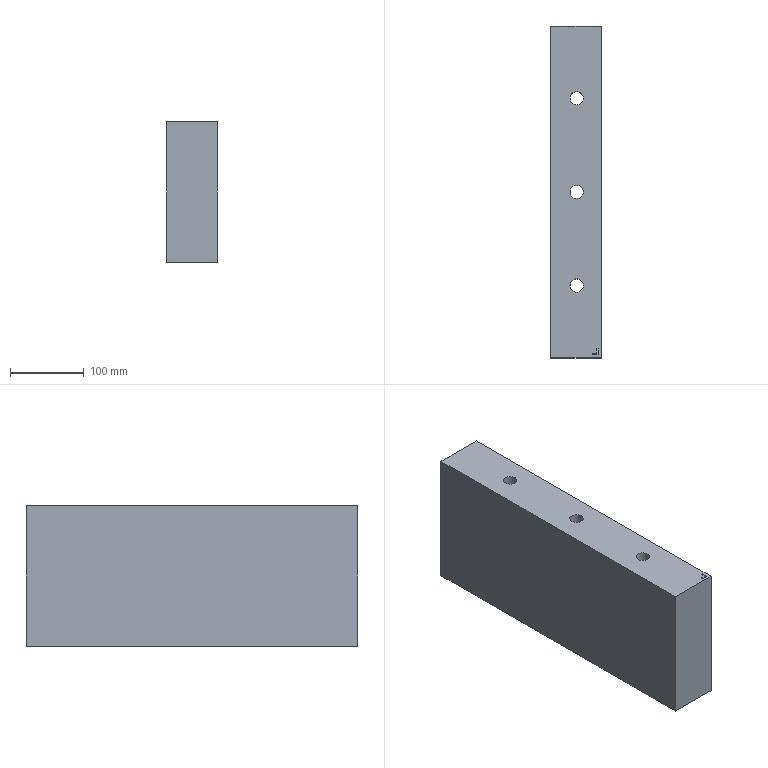Part | NX | features solid 2 | 1 solid | 32 faces | box 68 x 450 x 190 mm | volume 5663632 mm3 | plane 21 | cylinder 9 | cone 2 | commonest cylinder face diameters 18 x3 10.2 x2 11.7 x2 12 x2
STEP:
#1=CARTESIAN_POINT('',(-174.,127.,-380.5));
#2=VERTEX_POINT('',#1);
#3=CARTESIAN_POINT('',(-165.,127.,-380.5));
#4=DIRECTION('',(0.,0.,-1.));
#5=DIRECTION('',(-1.,0.,0.));
#6=AXIS2_PLACEMENT_3D('',#3,#4,#5);
#7=CIRCLE('',#6,9.);
#8=EDGE_CURVE('',#2,#2,#7,.T.);
#9=ORIENTED_EDGE('',*,*,#8,.F.);
#10=EDGE_LOOP('',(#9));
#11=FACE_BOUND('',#10,.T.);
#12=CARTESIAN_POINT('',(-174.,0.,-380.5));
#13=VERTEX_POINT('',#12);
#14=CARTESIAN_POINT('',(-165.,0.,-380.5));
#15=DIRECTION('',(0.,0.,-1.));
#16=DIRECTION('',(-1.,0.,0.));
#17=AXIS2_PLACEMENT_3D('',#14,#15,#16);
#18=CIRCLE('',#17,9.);
#19=EDGE_CURVE('',#13,#13,#18,.T.);
#20=ORIENTED_EDGE('',*,*,#19,.F.);
#21=EDGE_LOOP('',(#20));
#22=FACE_BOUND('',#21,.T.);
#23=CARTESIAN_POINT('',(-174.,-127.,-380.5));
#24=VERTEX_POINT('',#23);
#25=CARTESIAN_POINT('',(-165.,-127.,-380.5));
#26=DIRECTION('',(0.,0.,-1.));
#27=DIRECTION('',(-1.,0.,0.));
#28=AXIS2_PLACEMENT_3D('',#25,#26,#27);
#29=CIRCLE('',#28,9.);
#30=EDGE_CURVE('',#24,#24,#29,.T.);
#31=ORIENTED_EDGE('',*,*,#30,.F.);
#32=EDGE_LOOP('',(#31));
#33=FACE_BOUND('',#32,.T.);
#34=CARTESIAN_POINT('',(-170.1,187.,-380.5));
#35=VERTEX_POINT('',#34);
#36=CARTESIAN_POINT('',(-165.,187.,-380.5));
#37=DIRECTION('',(0.,0.,-1.));
#38=DIRECTION('',(-1.,0.,0.));
#39=AXIS2_PLACEMENT_3D('',#36,#37,#38);
#40=CIRCLE('',#39,5.1);
#41=EDGE_CURVE('',#35,#35,#40,.T.);
#42=ORIENTED_EDGE('',*,*,#41,.F.);
#43=EDGE_LOOP('',(#42));
#44=FACE_BOUND('',#43,.T.);
#45=CARTESIAN_POINT('',(-170.1,-187.,-380.5));
#46=VERTEX_POINT('',#45);
#47=CARTESIAN_POINT('',(-165.,-187.,-380.5));
#48=DIRECTION('',(0.,0.,-1.));
#49=DIRECTION('',(-1.,0.,0.));
#50=AXIS2_PLACEMENT_3D('',#47,#48,#49);
#51=CIRCLE('',#50,5.1);
#52=EDGE_CURVE('',#46,#46,#51,.T.);
#53=ORIENTED_EDGE('',*,*,#52,.F.);
#54=EDGE_LOOP('',(#53));
#55=FACE_BOUND('',#54,.T.);
#56=CARTESIAN_POINT('',(-132.,-225.,-380.5));
#57=VERTEX_POINT('',#56);
#58=CARTESIAN_POINT('',(-132.,225.,-380.5));
#59=VERTEX_POINT('',#58);
#60=CARTESIAN_POINT('',(-132.,0.,-380.5));
#61=DIRECTION('',(0.,1.,0.));
#62=VECTOR('',#61,1000.);
#63=LINE('',#60,#62);
#64=EDGE_CURVE('',#57,#59,#63,.T.);
#65=ORIENTED_EDGE('',*,*,#64,.F.);
#66=CARTESIAN_POINT('',(-200.,-225.,-380.5));
#67=VERTEX_POINT('',#66);
#68=CARTESIAN_POINT('',(-166.,-225.,-380.5));
#69=DIRECTION('',(1.,0.,0.));
#70=VECTOR('',#69,1000.);
#71=LINE('',#68,#70);
#72=EDGE_CURVE('',#67,#57,#71,.T.);
#73=ORIENTED_EDGE('',*,*,#72,.F.);
#74=CARTESIAN_POINT('',(-200.,225.,-380.5));
#75=VERTEX_POINT('',#74);
#76=CARTESIAN_POINT('',(-200.,0.,-380.5));
#77=DIRECTION('',(0.,-1.,0.));
#78=VECTOR('',#77,1000.);
#79=LINE('',#76,#78);
#80=EDGE_CURVE('',#75,#67,#79,.T.);
#81=ORIENTED_EDGE('',*,*,#80,.F.);
#82=CARTESIAN_POINT('',(-166.,225.,-380.5));
#83=DIRECTION('',(-1.,0.,0.));
#84=VECTOR('',#83,1000.);
#85=LINE('',#82,#84);
#86=EDGE_CURVE('',#59,#75,#85,.T.);
#87=ORIENTED_EDGE('',*,*,#86,.F.);
#88=EDGE_LOOP('',(#65,#73,#81,#87));
#89=FACE_BOUND('',#88,.T.);
#90=CARTESIAN_POINT('',(-165.,-192.85,-380.5));
#91=VERTEX_POINT('',#90);
#92=CARTESIAN_POINT('',(-159.15,-187.,-380.5));
#93=VERTEX_POINT('',#92);
#94=CARTESIAN_POINT('',(-165.,-187.,-380.5));
#95=DIRECTION('',(0.,0.,-1.));
#96=DIRECTION('',(-1.,0.,0.));
#97=AXIS2_PLACEMENT_3D('',#94,#95,#96);
#98=CIRCLE('',#97,5.85);
#99=EDGE_CURVE('',#91,#93,#98,.T.);
#100=ORIENTED_EDGE('',*,*,#99,.T.);
#101=CARTESIAN_POINT('',(-159.,-187.,-380.5));
#102=VERTEX_POINT('',#101);
#103=CARTESIAN_POINT('',(-166.,-187.,-380.5));
#104=DIRECTION('',(1.,0.,0.));
#105=VECTOR('',#104,1000.);
#106=LINE('',#103,#105);
#107=EDGE_CURVE('',#93,#102,#106,.T.);
#108=ORIENTED_EDGE('',*,*,#107,.T.);
#109=CARTESIAN_POINT('',(-165.,-193.,-380.5));
#110=VERTEX_POINT('',#109);
#111=CARTESIAN_POINT('',(-165.,-187.,-380.5));
#112=DIRECTION('',(0.,0.,-1.));
#113=DIRECTION('',(-1.,0.,0.));
#114=AXIS2_PLACEMENT_3D('',#111,#112,#113);
#115=CIRCLE('',#114,6.);
#116=EDGE_CURVE('',#110,#102,#115,.T.);
#117=ORIENTED_EDGE('',*,*,#116,.F.);
#118=CARTESIAN_POINT('',(-165.,0.,-380.5));
#119=DIRECTION('',(0.,1.,0.));
#120=VECTOR('',#119,1000.);
#121=LINE('',#118,#120);
#122=EDGE_CURVE('',#110,#91,#121,.T.);
#123=ORIENTED_EDGE('',*,*,#122,.T.);
#124=EDGE_LOOP('',(#100,#108,#117,#123));
#125=FACE_BOUND('',#124,.T.);
#126=CARTESIAN_POINT('',(-165.,181.15,-380.5));
#127=VERTEX_POINT('',#126);
#128=CARTESIAN_POINT('',(-159.15,187.,-380.5));
#129=VERTEX_POINT('',#128);
#130=CARTESIAN_POINT('',(-165.,187.,-380.5));
#131=DIRECTION('',(0.,0.,-1.));
#132=DIRECTION('',(-1.,0.,0.));
#133=AXIS2_PLACEMENT_3D('',#130,#131,#132);
#134=CIRCLE('',#133,5.85);
#135=EDGE_CURVE('',#127,#129,#134,.T.);
#136=ORIENTED_EDGE('',*,*,#135,.T.);
#137=CARTESIAN_POINT('',(-159.,187.,-380.5));
#138=VERTEX_POINT('',#137);
#139=CARTESIAN_POINT('',(-166.,187.,-380.5));
#140=DIRECTION('',(1.,0.,0.));
#141=VECTOR('',#140,1000.);
#142=LINE('',#139,#141);
#143=EDGE_CURVE('',#129,#138,#142,.T.);
#144=ORIENTED_EDGE('',*,*,#143,.T.);
#145=CARTESIAN_POINT('',(-165.,181.,-380.5));
#146=VERTEX_POINT('',#145);
#147=CARTESIAN_POINT('',(-165.,187.,-380.5));
#148=DIRECTION('',(0.,0.,-1.));
#149=DIRECTION('',(-1.,0.,0.));
#150=AXIS2_PLACEMENT_3D('',#147,#148,#149);
#151=CIRCLE('',#150,6.);
#152=EDGE_CURVE('',#146,#138,#151,.T.);
#153=ORIENTED_EDGE('',*,*,#152,.F.);
#154=CARTESIAN_POINT('',(-165.,0.,-380.5));
#155=DIRECTION('',(0.,1.,0.));
#156=VECTOR('',#155,1000.);
#157=LINE('',#154,#156);
#158=EDGE_CURVE('',#146,#127,#157,.T.);
#159=ORIENTED_EDGE('',*,*,#158,.T.);
#160=EDGE_LOOP('',(#136,#144,#153,#159));
#161=FACE_BOUND('',#160,.T.);
#162=CARTESIAN_POINT('',(-166.,0.,-380.5));
#163=DIRECTION('',(0.,0.,-1.));
#164=DIRECTION('',(-1.,0.,0.));
#165=AXIS2_PLACEMENT_3D('',#162,#163,#164);
#166=PLANE('',#165);
#167=ADVANCED_FACE('',(#11,#22,#33,#44,#55,#89,#125,#161),#166,.T.);
#168=CARTESIAN_POINT('',(-156.,127.,-190.5));
#169=VERTEX_POINT('',#168);
#170=CARTESIAN_POINT('',(-165.,127.,-190.5));
#171=DIRECTION('',(0.,0.,-1.));
#172=DIRECTION('',(1.,0.,0.));
#173=AXIS2_PLACEMENT_3D('',#170,#171,#172);
#174=CIRCLE('',#173,9.);
#175=EDGE_CURVE('',#169,#169,#174,.T.);
#176=ORIENTED_EDGE('',*,*,#175,.T.);
#177=EDGE_LOOP('',(#176));
#178=FACE_BOUND('',#177,.T.);
#179=CARTESIAN_POINT('',(-156.,0.,-190.5));
#180=VERTEX_POINT('',#179);
#181=CARTESIAN_POINT('',(-165.,0.,-190.5));
#182=DIRECTION('',(0.,0.,-1.));
#183=DIRECTION('',(1.,0.,0.));
#184=AXIS2_PLACEMENT_3D('',#181,#182,#183);
#185=CIRCLE('',#184,9.);
#186=EDGE_CURVE('',#180,#180,#185,.T.);
#187=ORIENTED_EDGE('',*,*,#186,.T.);
#188=EDGE_LOOP('',(#187));
#189=FACE_BOUND('',#188,.T.);
#190=CARTESIAN_POINT('',(-156.,-127.,-190.5));
#191=VERTEX_POINT('',#190);
#192=CARTESIAN_POINT('',(-165.,-127.,-190.5));
#193=DIRECTION('',(0.,0.,-1.));
#194=DIRECTION('',(1.,0.,0.));
#195=AXIS2_PLACEMENT_3D('',#192,#193,#194);
#196=CIRCLE('',#195,9.);
#197=EDGE_CURVE('',#191,#191,#196,.T.);
#198=ORIENTED_EDGE('',*,*,#197,.T.);
#199=EDGE_LOOP('',(#198));
#200=FACE_BOUND('',#199,.T.);
#201=CARTESIAN_POINT('',(-144.,-221.,-190.5));
#202=VERTEX_POINT('',#201);
#203=CARTESIAN_POINT('',(-136.,-221.,-190.5));
#204=VERTEX_POINT('',#203);
#205=CARTESIAN_POINT('',(-144.,-221.,-190.5));
#206=DIRECTION('',(1.,0.,0.));
#207=VECTOR('',#206,1000.);
#208=LINE('',#205,#207);
#209=EDGE_CURVE('',#202,#204,#208,.T.);
#210=ORIENTED_EDGE('',*,*,#209,.F.);
#211=CARTESIAN_POINT('',(-144.,-218.6,-190.5));
#212=VERTEX_POINT('',#211);
#213=CARTESIAN_POINT('',(-144.,-221.,-190.5));
#214=DIRECTION('',(0.,-1.,0.));
#215=VECTOR('',#214,1000.);
#216=LINE('',#213,#215);
#217=EDGE_CURVE('',#212,#202,#216,.T.);
#218=ORIENTED_EDGE('',*,*,#217,.F.);
#219=CARTESIAN_POINT('',(-138.4,-218.6,-190.5));
#220=VERTEX_POINT('',#219);
#221=CARTESIAN_POINT('',(-144.,-218.6,-190.5));
#222=DIRECTION('',(-1.,0.,0.));
#223=VECTOR('',#222,1000.);
#224=LINE('',#221,#223);
#225=EDGE_CURVE('',#220,#212,#224,.T.);
#226=ORIENTED_EDGE('',*,*,#225,.F.);
#227=CARTESIAN_POINT('',(-138.4,-213.,-190.5));
#228=VERTEX_POINT('',#227);
#229=CARTESIAN_POINT('',(-138.4,-218.6,-190.5));
#230=DIRECTION('',(0.,-1.,0.));
#231=VECTOR('',#230,1000.);
#232=LINE('',#229,#231);
#233=EDGE_CURVE('',#228,#220,#232,.T.);
#234=ORIENTED_EDGE('',*,*,#233,.F.);
#235=CARTESIAN_POINT('',(-136.,-213.,-190.5));
#236=VERTEX_POINT('',#235);
#237=CARTESIAN_POINT('',(-138.4,-213.,-190.5));
#238=DIRECTION('',(-1.,0.,0.));
#239=VECTOR('',#238,1000.);
#240=LINE('',#237,#239);
#241=EDGE_CURVE('',#236,#228,#240,.T.);
#242=ORIENTED_EDGE('',*,*,#241,.F.);
#243=CARTESIAN_POINT('',(-136.,-213.,-190.5));
#244=DIRECTION('',(0.,1.,0.));
#245=VECTOR('',#244,1000.);
#246=LINE('',#243,#245);
#247=EDGE_CURVE('',#204,#236,#246,.T.);
#248=ORIENTED_EDGE('',*,*,#247,.F.);
#249=EDGE_LOOP('',(#210,#218,#226,#234,#242,#248));
#250=FACE_BOUND('',#249,.T.);
#251=CARTESIAN_POINT('',(-132.,-225.,-190.5));
#252=VERTEX_POINT('',#251);
#253=CARTESIAN_POINT('',(-200.,-225.,-190.5));
#254=VERTEX_POINT('',#253);
#255=CARTESIAN_POINT('',(-166.,-225.,-190.5));
#256=DIRECTION('',(-1.,0.,0.));
#257=VECTOR('',#256,1000.);
#258=LINE('',#255,#257);
#259=EDGE_CURVE('',#252,#254,#258,.T.);
#260=ORIENTED_EDGE('',*,*,#259,.F.);
#261=CARTESIAN_POINT('',(-132.,225.,-190.5));
#262=VERTEX_POINT('',#261);
#263=CARTESIAN_POINT('',(-132.,0.,-190.5));
#264=DIRECTION('',(0.,-1.,0.));
#265=VECTOR('',#264,1000.);
#266=LINE('',#263,#265);
#267=EDGE_CURVE('',#262,#252,#266,.T.);
#268=ORIENTED_EDGE('',*,*,#267,.F.);
#269=CARTESIAN_POINT('',(-200.,225.,-190.5));
#270=VERTEX_POINT('',#269);
#271=CARTESIAN_POINT('',(-166.,225.,-190.5));
#272=DIRECTION('',(1.,0.,0.));
#273=VECTOR('',#272,1000.);
#274=LINE('',#271,#273);
#275=EDGE_CURVE('',#270,#262,#274,.T.);
#276=ORIENTED_EDGE('',*,*,#275,.F.);
#277=CARTESIAN_POINT('',(-200.,0.,-190.5));
#278=DIRECTION('',(0.,1.,0.));
#279=VECTOR('',#278,1000.);
#280=LINE('',#277,#279);
#281=EDGE_CURVE('',#254,#270,#280,.T.);
#282=ORIENTED_EDGE('',*,*,#281,.F.);
#283=EDGE_LOOP('',(#260,#268,#276,#282));
#284=FACE_BOUND('',#283,.T.);
#285=CARTESIAN_POINT('',(-166.,0.,-190.5));
#286=DIRECTION('',(0.,0.,1.));
#287=DIRECTION('',(1.,0.,0.));
#288=AXIS2_PLACEMENT_3D('',#285,#286,#287);
#289=PLANE('',#288);
#290=ADVANCED_FACE('',(#178,#189,#200,#250,#284),#289,.T.);
#291=CARTESIAN_POINT('',(-132.,-225.,-380.5));
#292=DIRECTION('',(0.,0.,1.));
#293=VECTOR('',#292,1000.);
#294=LINE('',#291,#293);
#295=EDGE_CURVE('',#57,#252,#294,.T.);
#296=ORIENTED_EDGE('',*,*,#295,.T.);
#297=ORIENTED_EDGE('',*,*,#259,.T.);
#298=CARTESIAN_POINT('',(-200.,-225.,-380.5));
#299=DIRECTION('',(0.,0.,1.));
#300=VECTOR('',#299,1000.);
#301=LINE('',#298,#300);
#302=EDGE_CURVE('',#67,#254,#301,.T.);
#303=ORIENTED_EDGE('',*,*,#302,.F.);
#304=ORIENTED_EDGE('',*,*,#72,.T.);
#305=EDGE_LOOP('',(#296,#297,#303,#304));
#306=FACE_BOUND('',#305,.T.);
#307=CARTESIAN_POINT('',(-166.,-225.,-380.5));
#308=DIRECTION('',(0.,-1.,0.));
#309=DIRECTION('',(0.,0.,-1.));
#310=AXIS2_PLACEMENT_3D('',#307,#308,#309);
#311=PLANE('',#310);
#312=ADVANCED_FACE('',(#306),#311,.T.);
#313=ORIENTED_EDGE('',*,*,#302,.T.);
#314=ORIENTED_EDGE('',*,*,#281,.T.);
#315=CARTESIAN_POINT('',(-200.,225.,-380.5));
#316=DIRECTION('',(0.,0.,1.));
#317=VECTOR('',#316,1000.);
#318=LINE('',#315,#317);
#319=EDGE_CURVE('',#75,#270,#318,.T.);
#320=ORIENTED_EDGE('',*,*,#319,.F.);
#321=ORIENTED_EDGE('',*,*,#80,.T.);
#322=EDGE_LOOP('',(#313,#314,#320,#321));
#323=FACE_BOUND('',#322,.T.);
#324=CARTESIAN_POINT('',(-200.,0.,-380.5));
#325=DIRECTION('',(-1.,0.,0.));
#326=DIRECTION('',(0.,0.,1.));
#327=AXIS2_PLACEMENT_3D('',#324,#325,#326);
#328=PLANE('',#327);
#329=ADVANCED_FACE('',(#323),#328,.T.);
#330=ORIENTED_EDGE('',*,*,#319,.T.);
#331=ORIENTED_EDGE('',*,*,#275,.T.);
#332=CARTESIAN_POINT('',(-132.,225.,-380.5));
#333=DIRECTION('',(0.,0.,1.));
#334=VECTOR('',#333,1000.);
#335=LINE('',#332,#334);
#336=EDGE_CURVE('',#59,#262,#335,.T.);
#337=ORIENTED_EDGE('',*,*,#336,.F.);
#338=ORIENTED_EDGE('',*,*,#86,.T.);
#339=EDGE_LOOP('',(#330,#331,#337,#338));
#340=FACE_BOUND('',#339,.T.);
#341=CARTESIAN_POINT('',(-166.,225.,-380.5));
#342=DIRECTION('',(0.,1.,0.));
#343=DIRECTION('',(0.,0.,1.));
#344=AXIS2_PLACEMENT_3D('',#341,#342,#343);
#345=PLANE('',#344);
#346=ADVANCED_FACE('',(#340),#345,.T.);
#347=ORIENTED_EDGE('',*,*,#64,.T.);
#348=ORIENTED_EDGE('',*,*,#336,.T.);
#349=ORIENTED_EDGE('',*,*,#267,.T.);
#350=ORIENTED_EDGE('',*,*,#295,.F.);
#351=EDGE_LOOP('',(#347,#348,#349,#350));
#352=FACE_BOUND('',#351,.T.);
#353=CARTESIAN_POINT('',(-132.,0.,-380.5));
#354=DIRECTION('',(1.,0.,0.));
#355=DIRECTION('',(0.,0.,-1.));
#356=AXIS2_PLACEMENT_3D('',#353,#354,#355);
#357=PLANE('',#356);
#358=ADVANCED_FACE('',(#352),#357,.T.);
#359=ORIENTED_EDGE('',*,*,#209,.T.);
#360=CARTESIAN_POINT('',(-136.,-221.,-190.8));
#361=VERTEX_POINT('',#360);
#362=CARTESIAN_POINT('',(-136.,-221.,-190.8));
#363=DIRECTION('',(0.,0.,1.));
#364=VECTOR('',#363,1000.);
#365=LINE('',#362,#364);
#366=EDGE_CURVE('',#361,#204,#365,.T.);
#367=ORIENTED_EDGE('',*,*,#366,.F.);
#368=CARTESIAN_POINT('',(-144.,-221.,-190.8));
#369=VERTEX_POINT('',#368);
#370=CARTESIAN_POINT('',(-144.,-221.,-190.8));
#371=DIRECTION('',(1.,0.,0.));
#372=VECTOR('',#371,1000.);
#373=LINE('',#370,#372);
#374=EDGE_CURVE('',#369,#361,#373,.T.);
#375=ORIENTED_EDGE('',*,*,#374,.F.);
#376=CARTESIAN_POINT('',(-144.,-221.,-190.8));
#377=DIRECTION('',(0.,0.,1.));
#378=VECTOR('',#377,1000.);
#379=LINE('',#376,#378);
#380=EDGE_CURVE('',#369,#202,#379,.T.);
#381=ORIENTED_EDGE('',*,*,#380,.T.);
#382=EDGE_LOOP('',(#359,#367,#375,#381));
#383=FACE_BOUND('',#382,.T.);
#384=CARTESIAN_POINT('',(-144.,-221.,-190.8));
#385=DIRECTION('',(0.,-1.,0.));
#386=DIRECTION('',(0.,0.,-1.));
#387=AXIS2_PLACEMENT_3D('',#384,#385,#386);
#388=PLANE('',#387);
#389=ADVANCED_FACE('',(#383),#388,.F.);
#390=ORIENTED_EDGE('',*,*,#247,.T.);
#391=CARTESIAN_POINT('',(-136.,-213.,-190.8));
#392=VERTEX_POINT('',#391);
#393=CARTESIAN_POINT('',(-136.,-213.,-190.8));
#394=DIRECTION('',(0.,0.,1.));
#395=VECTOR('',#394,1000.);
#396=LINE('',#393,#395);
#397=EDGE_CURVE('',#392,#236,#396,.T.);
#398=ORIENTED_EDGE('',*,*,#397,.F.);
#399=CARTESIAN_POINT('',(-136.,-213.,-190.8));
#400=DIRECTION('',(0.,1.,0.));
#401=VECTOR('',#400,1000.);
#402=LINE('',#399,#401);
#403=EDGE_CURVE('',#361,#392,#402,.T.);
#404=ORIENTED_EDGE('',*,*,#403,.F.);
#405=ORIENTED_EDGE('',*,*,#366,.T.);
#406=EDGE_LOOP('',(#390,#398,#404,#405));
#407=FACE_BOUND('',#406,.T.);
#408=CARTESIAN_POINT('',(-136.,-213.,-190.8));
#409=DIRECTION('',(1.,0.,0.));
#410=DIRECTION('',(0.,0.,-1.));
#411=AXIS2_PLACEMENT_3D('',#408,#409,#410);
#412=PLANE('',#411);
#413=ADVANCED_FACE('',(#407),#412,.F.);
#414=ORIENTED_EDGE('',*,*,#241,.T.);
#415=CARTESIAN_POINT('',(-138.4,-213.,-190.8));
#416=VERTEX_POINT('',#415);
#417=CARTESIAN_POINT('',(-138.4,-213.,-190.8));
#418=DIRECTION('',(0.,0.,1.));
#419=VECTOR('',#418,1000.);
#420=LINE('',#417,#419);
#421=EDGE_CURVE('',#416,#228,#420,.T.);
#422=ORIENTED_EDGE('',*,*,#421,.F.);
#423=CARTESIAN_POINT('',(-138.4,-213.,-190.8));
#424=DIRECTION('',(-1.,0.,0.));
#425=VECTOR('',#424,1000.);
#426=LINE('',#423,#425);
#427=EDGE_CURVE('',#392,#416,#426,.T.);
#428=ORIENTED_EDGE('',*,*,#427,.F.);
#429=ORIENTED_EDGE('',*,*,#397,.T.);
#430=EDGE_LOOP('',(#414,#422,#428,#429));
#431=FACE_BOUND('',#430,.T.);
#432=CARTESIAN_POINT('',(-138.4,-213.,-190.8));
#433=DIRECTION('',(0.,1.,0.));
#434=DIRECTION('',(0.,0.,1.));
#435=AXIS2_PLACEMENT_3D('',#432,#433,#434);
#436=PLANE('',#435);
#437=ADVANCED_FACE('',(#431),#436,.F.);
#438=ORIENTED_EDGE('',*,*,#233,.T.);
#439=CARTESIAN_POINT('',(-138.4,-218.6,-190.8));
#440=VERTEX_POINT('',#439);
#441=CARTESIAN_POINT('',(-138.4,-218.6,-190.8));
#442=DIRECTION('',(0.,0.,1.));
#443=VECTOR('',#442,1000.);
#444=LINE('',#441,#443);
#445=EDGE_CURVE('',#440,#220,#444,.T.);
#446=ORIENTED_EDGE('',*,*,#445,.F.);
#447=CARTESIAN_POINT('',(-138.4,-218.6,-190.8));
#448=DIRECTION('',(0.,-1.,0.));
#449=VECTOR('',#448,1000.);
#450=LINE('',#447,#449);
#451=EDGE_CURVE('',#416,#440,#450,.T.);
#452=ORIENTED_EDGE('',*,*,#451,.F.);
#453=ORIENTED_EDGE('',*,*,#421,.T.);
#454=EDGE_LOOP('',(#438,#446,#452,#453));
#455=FACE_BOUND('',#454,.T.);
#456=CARTESIAN_POINT('',(-138.4,-218.6,-190.8));
#457=DIRECTION('',(-1.,0.,0.));
#458=DIRECTION('',(0.,0.,1.));
#459=AXIS2_PLACEMENT_3D('',#456,#457,#458);
#460=PLANE('',#459);
#461=ADVANCED_FACE('',(#455),#460,.F.);
#462=ORIENTED_EDGE('',*,*,#225,.T.);
#463=CARTESIAN_POINT('',(-144.,-218.6,-190.8));
#464=VERTEX_POINT('',#463);
#465=CARTESIAN_POINT('',(-144.,-218.6,-190.8));
#466=DIRECTION('',(0.,0.,1.));
#467=VECTOR('',#466,1000.);
#468=LINE('',#465,#467);
#469=EDGE_CURVE('',#464,#212,#468,.T.);
#470=ORIENTED_EDGE('',*,*,#469,.F.);
#471=CARTESIAN_POINT('',(-144.,-218.6,-190.8));
#472=DIRECTION('',(-1.,0.,0.));
#473=VECTOR('',#472,1000.);
#474=LINE('',#471,#473);
#475=EDGE_CURVE('',#440,#464,#474,.T.);
#476=ORIENTED_EDGE('',*,*,#475,.F.);
#477=ORIENTED_EDGE('',*,*,#445,.T.);
#478=EDGE_LOOP('',(#462,#470,#476,#477));
#479=FACE_BOUND('',#478,.T.);
#480=CARTESIAN_POINT('',(-144.,-218.6,-190.8));
#481=DIRECTION('',(0.,1.,0.));
#482=DIRECTION('',(0.,0.,1.));
#483=AXIS2_PLACEMENT_3D('',#480,#481,#482);
#484=PLANE('',#483);
#485=ADVANCED_FACE('',(#479),#484,.F.);
#486=ORIENTED_EDGE('',*,*,#217,.T.);
#487=ORIENTED_EDGE('',*,*,#380,.F.);
#488=CARTESIAN_POINT('',(-144.,-221.,-190.8));
#489=DIRECTION('',(0.,-1.,0.));
#490=VECTOR('',#489,1000.);
#491=LINE('',#488,#490);
#492=EDGE_CURVE('',#464,#369,#491,.T.);
#493=ORIENTED_EDGE('',*,*,#492,.F.);
#494=ORIENTED_EDGE('',*,*,#469,.T.);
#495=EDGE_LOOP('',(#486,#487,#493,#494));
#496=FACE_BOUND('',#495,.T.);
#497=CARTESIAN_POINT('',(-144.,-221.,-190.8));
#498=DIRECTION('',(-1.,0.,0.));
#499=DIRECTION('',(0.,0.,1.));
#500=AXIS2_PLACEMENT_3D('',#497,#498,#499);
#501=PLANE('',#500);
#502=ADVANCED_FACE('',(#496),#501,.F.);
#503=ORIENTED_EDGE('',*,*,#374,.T.);
#504=ORIENTED_EDGE('',*,*,#403,.T.);
#505=ORIENTED_EDGE('',*,*,#427,.T.);
#506=ORIENTED_EDGE('',*,*,#451,.T.);
#507=ORIENTED_EDGE('',*,*,#475,.T.);
#508=ORIENTED_EDGE('',*,*,#492,.T.);
#509=EDGE_LOOP('',(#503,#504,#505,#506,#507,#508));
#510=FACE_BOUND('',#509,.T.);
#511=CARTESIAN_POINT('',(-136.,-221.,-190.8));
#512=DIRECTION('',(0.,0.,1.));
#513=DIRECTION('',(1.,0.,0.));
#514=AXIS2_PLACEMENT_3D('',#511,#512,#513);
#515=PLANE('',#514);
#516=ADVANCED_FACE('',(#510),#515,.T.);
#517=CARTESIAN_POINT('',(-159.9,-187.,-356.5));
#518=VERTEX_POINT('',#517);
#519=CARTESIAN_POINT('',(-165.,-192.1,-356.5));
#520=VERTEX_POINT('',#519);
#521=CARTESIAN_POINT('',(-165.,-187.,-356.5));
#522=DIRECTION('',(0.,0.,1.));
#523=DIRECTION('',(0.,-1.,0.));
#524=AXIS2_PLACEMENT_3D('',#521,#522,#523);
#525=CIRCLE('',#524,5.1);
#526=EDGE_CURVE('',#518,#520,#525,.T.);
#527=ORIENTED_EDGE('',*,*,#526,.T.);
#528=CARTESIAN_POINT('',(-165.,-193.,-356.5));
#529=VERTEX_POINT('',#528);
#530=CARTESIAN_POINT('',(-165.,-193.,-356.5));
#531=DIRECTION('',(0.,1.,0.));
#532=VECTOR('',#531,1000.);
#533=LINE('',#530,#532);
#534=EDGE_CURVE('',#529,#520,#533,.T.);
#535=ORIENTED_EDGE('',*,*,#534,.F.);
#536=CARTESIAN_POINT('',(-159.,-187.,-356.5));
#537=VERTEX_POINT('',#536);
#538=CARTESIAN_POINT('',(-165.,-187.,-356.5));
#539=DIRECTION('',(0.,0.,-1.));
#540=DIRECTION('',(1.,0.,0.));
#541=AXIS2_PLACEMENT_3D('',#538,#539,#540);
#542=CIRCLE('',#541,6.);
#543=EDGE_CURVE('',#529,#537,#542,.T.);
#544=ORIENTED_EDGE('',*,*,#543,.T.);
#545=CARTESIAN_POINT('',(-159.,-187.,-356.5));
#546=DIRECTION('',(1.,0.,0.));
#547=VECTOR('',#546,1000.);
#548=LINE('',#545,#547);
#549=EDGE_CURVE('',#518,#537,#548,.T.);
#550=ORIENTED_EDGE('',*,*,#549,.F.);
#551=EDGE_LOOP('',(#527,#535,#544,#550));
#552=FACE_BOUND('',#551,.T.);
#553=CARTESIAN_POINT('',(-165.,-187.,-356.5));
#554=DIRECTION('',(0.,0.,1.));
#555=DIRECTION('',(0.,-1.,0.));
#556=AXIS2_PLACEMENT_3D('',#553,#554,#555);
#557=PLANE('',#556);
#558=ADVANCED_FACE('',(#552),#557,.F.);
#559=ORIENTED_EDGE('',*,*,#116,.T.);
#560=CARTESIAN_POINT('',(-159.,-187.,-356.5));
#561=DIRECTION('',(0.,0.,-1.));
#562=VECTOR('',#561,1000.);
#563=LINE('',#560,#562);
#564=EDGE_CURVE('',#102,#537,#563,.F.);
#565=ORIENTED_EDGE('',*,*,#564,.T.);
#566=ORIENTED_EDGE('',*,*,#543,.F.);
#567=CARTESIAN_POINT('',(-165.,-193.,-356.5));
#568=DIRECTION('',(0.,0.,-1.));
#569=VECTOR('',#568,1000.);
#570=LINE('',#567,#569);
#571=EDGE_CURVE('',#529,#110,#570,.T.);
#572=ORIENTED_EDGE('',*,*,#571,.T.);
#573=EDGE_LOOP('',(#559,#565,#566,#572));
#574=FACE_BOUND('',#573,.T.);
#575=CARTESIAN_POINT('',(-165.,-187.,-356.5));
#576=DIRECTION('',(0.,0.,-1.));
#577=DIRECTION('',(1.,0.,0.));
#578=AXIS2_PLACEMENT_3D('',#575,#576,#577);
#579=CYLINDRICAL_SURFACE('',#578,6.);
#580=ADVANCED_FACE('',(#574),#579,.F.);
#581=CARTESIAN_POINT('',(-159.15,-187.,-357.5));
#582=VERTEX_POINT('',#581);
#583=CARTESIAN_POINT('',(-159.9,-187.,-357.5));
#584=VERTEX_POINT('',#583);
#585=CARTESIAN_POINT('',(-165.,-187.,-357.5));
#586=DIRECTION('',(-1.,0.,0.));
#587=VECTOR('',#586,1000.);
#588=LINE('',#585,#587);
#589=EDGE_CURVE('',#582,#584,#588,.T.);
#590=ORIENTED_EDGE('',*,*,#589,.F.);
#591=CARTESIAN_POINT('',(-165.,-192.85,-357.5));
#592=VERTEX_POINT('',#591);
#593=CARTESIAN_POINT('',(-165.,-187.,-357.5));
#594=DIRECTION('',(0.,0.,-1.));
#595=DIRECTION('',(1.,0.,0.));
#596=AXIS2_PLACEMENT_3D('',#593,#594,#595);
#597=CIRCLE('',#596,5.85);
#598=EDGE_CURVE('',#592,#582,#597,.T.);
#599=ORIENTED_EDGE('',*,*,#598,.F.);
#600=CARTESIAN_POINT('',(-165.,-192.1,-357.5));
#601=VERTEX_POINT('',#600);
#602=CARTESIAN_POINT('',(-165.,-187.,-357.5));
#603=DIRECTION('',(0.,-1.,0.));
#604=VECTOR('',#603,1000.);
#605=LINE('',#602,#604);
#606=EDGE_CURVE('',#601,#592,#605,.T.);
#607=ORIENTED_EDGE('',*,*,#606,.F.);
#608=CARTESIAN_POINT('',(-165.,-187.,-357.5));
#609=DIRECTION('',(0.,0.,1.));
#610=DIRECTION('',(0.,-1.,0.));
#611=AXIS2_PLACEMENT_3D('',#608,#609,#610);
#612=CIRCLE('',#611,5.1);
#613=EDGE_CURVE('',#584,#601,#612,.T.);
#614=ORIENTED_EDGE('',*,*,#613,.F.);
#615=EDGE_LOOP('',(#590,#599,#607,#614));
#616=FACE_BOUND('',#615,.T.);
#617=CARTESIAN_POINT('',(-165.,-187.,-357.5));
#618=DIRECTION('',(0.,0.,1.));
#619=DIRECTION('',(0.,-1.,0.));
#620=AXIS2_PLACEMENT_3D('',#617,#618,#619);
#621=PLANE('',#620);
#622=ADVANCED_FACE('',(#616),#621,.T.);
#623=CARTESIAN_POINT('',(-165.,-192.85,-357.5));
#624=DIRECTION('',(0.,0.,-1.));
#625=VECTOR('',#624,1000.);
#626=LINE('',#623,#625);
#627=EDGE_CURVE('',#592,#91,#626,.T.);
#628=ORIENTED_EDGE('',*,*,#627,.F.);
#629=ORIENTED_EDGE('',*,*,#598,.T.);
#630=CARTESIAN_POINT('',(-159.15,-187.,-357.5));
#631=DIRECTION('',(0.,0.,-1.));
#632=VECTOR('',#631,1000.);
#633=LINE('',#630,#632);
#634=EDGE_CURVE('',#93,#582,#633,.F.);
#635=ORIENTED_EDGE('',*,*,#634,.F.);
#636=ORIENTED_EDGE('',*,*,#99,.F.);
#637=EDGE_LOOP('',(#628,#629,#635,#636));
#638=FACE_BOUND('',#637,.T.);
#639=CARTESIAN_POINT('',(-165.,-187.,-357.5));
#640=DIRECTION('',(0.,0.,-1.));
#641=DIRECTION('',(1.,0.,0.));
#642=AXIS2_PLACEMENT_3D('',#639,#640,#641);
#643=CYLINDRICAL_SURFACE('',#642,5.85);
#644=ADVANCED_FACE('',(#638),#643,.T.);
#645=ORIENTED_EDGE('',*,*,#634,.T.);
#646=ORIENTED_EDGE('',*,*,#589,.T.);
#647=CARTESIAN_POINT('',(-159.9,-187.,-350.449));
#648=DIRECTION('',(0.,0.,-1.));
#649=VECTOR('',#648,1000.);
#650=LINE('',#647,#649);
#651=EDGE_CURVE('',#518,#584,#650,.T.);
#652=ORIENTED_EDGE('',*,*,#651,.F.);
#653=ORIENTED_EDGE('',*,*,#549,.T.);
#654=ORIENTED_EDGE('',*,*,#564,.F.);
#655=ORIENTED_EDGE('',*,*,#107,.F.);
#656=EDGE_LOOP('',(#645,#646,#652,#653,#654,#655));
#657=FACE_BOUND('',#656,.T.);
#658=CARTESIAN_POINT('',(-159.,-187.,-356.5));
#659=DIRECTION('',(0.,1.,0.));
#660=DIRECTION('',(0.,0.,1.));
#661=AXIS2_PLACEMENT_3D('',#658,#659,#660);
#662=PLANE('',#661);
#663=ADVANCED_FACE('',(#657),#662,.T.);
#664=ORIENTED_EDGE('',*,*,#571,.F.);
#665=ORIENTED_EDGE('',*,*,#534,.T.);
#666=CARTESIAN_POINT('',(-165.,-192.1,-350.449));
#667=DIRECTION('',(0.,0.,-1.));
#668=VECTOR('',#667,1000.);
#669=LINE('',#666,#668);
#670=EDGE_CURVE('',#601,#520,#669,.F.);
#671=ORIENTED_EDGE('',*,*,#670,.F.);
#672=ORIENTED_EDGE('',*,*,#606,.T.);
#673=ORIENTED_EDGE('',*,*,#627,.T.);
#674=ORIENTED_EDGE('',*,*,#122,.F.);
#675=EDGE_LOOP('',(#664,#665,#671,#672,#673,#674));
#676=FACE_BOUND('',#675,.T.);
#677=CARTESIAN_POINT('',(-165.,-193.,-356.5));
#678=DIRECTION('',(-1.,0.,0.));
#679=DIRECTION('',(0.,0.,1.));
#680=AXIS2_PLACEMENT_3D('',#677,#678,#679);
#681=PLANE('',#680);
#682=ADVANCED_FACE('',(#676),#681,.T.);
#683=ORIENTED_EDGE('',*,*,#52,.T.);
#684=EDGE_LOOP('',(#683));
#685=FACE_BOUND('',#684,.T.);
#686=CARTESIAN_POINT('',(-159.9,-187.,-350.449));
#687=VERTEX_POINT('',#686);
#688=CARTESIAN_POINT('',(-165.,-187.,-350.449));
#689=DIRECTION('',(0.,0.,1.));
#690=DIRECTION('',(1.,0.,0.));
#691=AXIS2_PLACEMENT_3D('',#688,#689,#690);
#692=CIRCLE('',#691,5.1);
#693=EDGE_CURVE('',#687,#687,#692,.T.);
#694=ORIENTED_EDGE('',*,*,#693,.T.);
#695=EDGE_LOOP('',(#694));
#696=FACE_BOUND('',#695,.T.);
#697=ORIENTED_EDGE('',*,*,#651,.T.);
#698=ORIENTED_EDGE('',*,*,#613,.T.);
#699=ORIENTED_EDGE('',*,*,#670,.T.);
#700=ORIENTED_EDGE('',*,*,#526,.F.);
#701=EDGE_LOOP('',(#697,#698,#699,#700));
#702=FACE_BOUND('',#701,.T.);
#703=CARTESIAN_POINT('',(-165.,-187.,-350.449));
#704=DIRECTION('',(0.,0.,-1.));
#705=DIRECTION('',(1.,0.,0.));
#706=AXIS2_PLACEMENT_3D('',#703,#704,#705);
#707=CYLINDRICAL_SURFACE('',#706,5.1);
#708=ADVANCED_FACE('',(#685,#696,#702),#707,.F.);
#709=ORIENTED_EDGE('',*,*,#693,.F.);
#710=EDGE_LOOP('',(#709));
#711=FACE_BOUND('',#710,.T.);
#712=CARTESIAN_POINT('',(-165.,-187.,-347.505));
#713=VERTEX_POINT('',#712);
#714=VERTEX_LOOP('',#713);
#715=FACE_BOUND('',#714,.T.);
#716=CARTESIAN_POINT('',(-165.,-187.,-347.505));
#717=DIRECTION('',(0.,0.,-1.));
#718=DIRECTION('',(1.,0.,0.));
#719=AXIS2_PLACEMENT_3D('',#716,#717,#718);
#720=CONICAL_SURFACE('',#719,0.,1.047);
#721=ADVANCED_FACE('',(#711,#715),#720,.F.);
#722=CARTESIAN_POINT('',(-159.9,187.,-356.5));
#723=VERTEX_POINT('',#722);
#724=CARTESIAN_POINT('',(-165.,181.9,-356.5));
#725=VERTEX_POINT('',#724);
#726=CARTESIAN_POINT('',(-165.,187.,-356.5));
#727=DIRECTION('',(0.,0.,1.));
#728=DIRECTION('',(0.,-1.,0.));
#729=AXIS2_PLACEMENT_3D('',#726,#727,#728);
#730=CIRCLE('',#729,5.1);
#731=EDGE_CURVE('',#723,#725,#730,.T.);
#732=ORIENTED_EDGE('',*,*,#731,.T.);
#733=CARTESIAN_POINT('',(-165.,181.,-356.5));
#734=VERTEX_POINT('',#733);
#735=CARTESIAN_POINT('',(-165.,181.,-356.5));
#736=DIRECTION('',(0.,1.,0.));
#737=VECTOR('',#736,1000.);
#738=LINE('',#735,#737);
#739=EDGE_CURVE('',#734,#725,#738,.T.);
#740=ORIENTED_EDGE('',*,*,#739,.F.);
#741=CARTESIAN_POINT('',(-159.,187.,-356.5));
#742=VERTEX_POINT('',#741);
#743=CARTESIAN_POINT('',(-165.,187.,-356.5));
#744=DIRECTION('',(0.,0.,-1.));
#745=DIRECTION('',(1.,0.,0.));
#746=AXIS2_PLACEMENT_3D('',#743,#744,#745);
#747=CIRCLE('',#746,6.);
#748=EDGE_CURVE('',#734,#742,#747,.T.);
#749=ORIENTED_EDGE('',*,*,#748,.T.);
#750=CARTESIAN_POINT('',(-159.,187.,-356.5));
#751=DIRECTION('',(1.,0.,0.));
#752=VECTOR('',#751,1000.);
#753=LINE('',#750,#752);
#754=EDGE_CURVE('',#723,#742,#753,.T.);
#755=ORIENTED_EDGE('',*,*,#754,.F.);
#756=EDGE_LOOP('',(#732,#740,#749,#755));
#757=FACE_BOUND('',#756,.T.);
#758=CARTESIAN_POINT('',(-165.,187.,-356.5));
#759=DIRECTION('',(0.,0.,1.));
#760=DIRECTION('',(0.,-1.,0.));
#761=AXIS2_PLACEMENT_3D('',#758,#759,#760);
#762=PLANE('',#761);
#763=ADVANCED_FACE('',(#757),#762,.F.);
#764=ORIENTED_EDGE('',*,*,#152,.T.);
#765=CARTESIAN_POINT('',(-159.,187.,-356.5));
#766=DIRECTION('',(0.,0.,-1.));
#767=VECTOR('',#766,1000.);
#768=LINE('',#765,#767);
#769=EDGE_CURVE('',#138,#742,#768,.F.);
#770=ORIENTED_EDGE('',*,*,#769,.T.);
#771=ORIENTED_EDGE('',*,*,#748,.F.);
#772=CARTESIAN_POINT('',(-165.,181.,-356.5));
#773=DIRECTION('',(0.,0.,-1.));
#774=VECTOR('',#773,1000.);
#775=LINE('',#772,#774);
#776=EDGE_CURVE('',#734,#146,#775,.T.);
#777=ORIENTED_EDGE('',*,*,#776,.T.);
#778=EDGE_LOOP('',(#764,#770,#771,#777));
#779=FACE_BOUND('',#778,.T.);
#780=CARTESIAN_POINT('',(-165.,187.,-356.5));
#781=DIRECTION('',(0.,0.,-1.));
#782=DIRECTION('',(1.,0.,0.));
#783=AXIS2_PLACEMENT_3D('',#780,#781,#782);
#784=CYLINDRICAL_SURFACE('',#783,6.);
#785=ADVANCED_FACE('',(#779),#784,.F.);
#786=CARTESIAN_POINT('',(-159.15,187.,-357.5));
#787=VERTEX_POINT('',#786);
#788=CARTESIAN_POINT('',(-159.9,187.,-357.5));
#789=VERTEX_POINT('',#788);
#790=CARTESIAN_POINT('',(-165.,187.,-357.5));
#791=DIRECTION('',(-1.,0.,0.));
#792=VECTOR('',#791,1000.);
#793=LINE('',#790,#792);
#794=EDGE_CURVE('',#787,#789,#793,.T.);
#795=ORIENTED_EDGE('',*,*,#794,.F.);
#796=CARTESIAN_POINT('',(-165.,181.15,-357.5));
#797=VERTEX_POINT('',#796);
#798=CARTESIAN_POINT('',(-165.,187.,-357.5));
#799=DIRECTION('',(0.,0.,-1.));
#800=DIRECTION('',(1.,0.,0.));
#801=AXIS2_PLACEMENT_3D('',#798,#799,#800);
#802=CIRCLE('',#801,5.85);
#803=EDGE_CURVE('',#797,#787,#802,.T.);
#804=ORIENTED_EDGE('',*,*,#803,.F.);
#805=CARTESIAN_POINT('',(-165.,181.9,-357.5));
#806=VERTEX_POINT('',#805);
#807=CARTESIAN_POINT('',(-165.,187.,-357.5));
#808=DIRECTION('',(0.,-1.,0.));
#809=VECTOR('',#808,1000.);
#810=LINE('',#807,#809);
#811=EDGE_CURVE('',#806,#797,#810,.T.);
#812=ORIENTED_EDGE('',*,*,#811,.F.);
#813=CARTESIAN_POINT('',(-165.,187.,-357.5));
#814=DIRECTION('',(0.,0.,1.));
#815=DIRECTION('',(0.,-1.,0.));
#816=AXIS2_PLACEMENT_3D('',#813,#814,#815);
#817=CIRCLE('',#816,5.1);
#818=EDGE_CURVE('',#789,#806,#817,.T.);
#819=ORIENTED_EDGE('',*,*,#818,.F.);
#820=EDGE_LOOP('',(#795,#804,#812,#819));
#821=FACE_BOUND('',#820,.T.);
#822=CARTESIAN_POINT('',(-165.,187.,-357.5));
#823=DIRECTION('',(0.,0.,1.));
#824=DIRECTION('',(0.,-1.,0.));
#825=AXIS2_PLACEMENT_3D('',#822,#823,#824);
#826=PLANE('',#825);
#827=ADVANCED_FACE('',(#821),#826,.T.);
#828=CARTESIAN_POINT('',(-165.,181.15,-357.5));
#829=DIRECTION('',(0.,0.,-1.));
#830=VECTOR('',#829,1000.);
#831=LINE('',#828,#830);
#832=EDGE_CURVE('',#797,#127,#831,.T.);
#833=ORIENTED_EDGE('',*,*,#832,.F.);
#834=ORIENTED_EDGE('',*,*,#803,.T.);
#835=CARTESIAN_POINT('',(-159.15,187.,-357.5));
#836=DIRECTION('',(0.,0.,-1.));
#837=VECTOR('',#836,1000.);
#838=LINE('',#835,#837);
#839=EDGE_CURVE('',#129,#787,#838,.F.);
#840=ORIENTED_EDGE('',*,*,#839,.F.);
#841=ORIENTED_EDGE('',*,*,#135,.F.);
#842=EDGE_LOOP('',(#833,#834,#840,#841));
#843=FACE_BOUND('',#842,.T.);
#844=CARTESIAN_POINT('',(-165.,187.,-357.5));
#845=DIRECTION('',(0.,0.,-1.));
#846=DIRECTION('',(1.,0.,0.));
#847=AXIS2_PLACEMENT_3D('',#844,#845,#846);
#848=CYLINDRICAL_SURFACE('',#847,5.85);
#849=ADVANCED_FACE('',(#843),#848,.T.);
#850=ORIENTED_EDGE('',*,*,#839,.T.);
#851=ORIENTED_EDGE('',*,*,#794,.T.);
#852=CARTESIAN_POINT('',(-159.9,187.,-350.449));
#853=DIRECTION('',(0.,0.,-1.));
#854=VECTOR('',#853,1000.);
#855=LINE('',#852,#854);
#856=EDGE_CURVE('',#723,#789,#855,.T.);
#857=ORIENTED_EDGE('',*,*,#856,.F.);
#858=ORIENTED_EDGE('',*,*,#754,.T.);
#859=ORIENTED_EDGE('',*,*,#769,.F.);
#860=ORIENTED_EDGE('',*,*,#143,.F.);
#861=EDGE_LOOP('',(#850,#851,#857,#858,#859,#860));
#862=FACE_BOUND('',#861,.T.);
#863=CARTESIAN_POINT('',(-159.,187.,-356.5));
#864=DIRECTION('',(0.,1.,0.));
#865=DIRECTION('',(0.,0.,1.));
#866=AXIS2_PLACEMENT_3D('',#863,#864,#865);
#867=PLANE('',#866);
#868=ADVANCED_FACE('',(#862),#867,.T.);
#869=ORIENTED_EDGE('',*,*,#776,.F.);
#870=ORIENTED_EDGE('',*,*,#739,.T.);
#871=CARTESIAN_POINT('',(-165.,181.9,-350.449));
#872=DIRECTION('',(0.,0.,-1.));
#873=VECTOR('',#872,1000.);
#874=LINE('',#871,#873);
#875=EDGE_CURVE('',#806,#725,#874,.F.);
#876=ORIENTED_EDGE('',*,*,#875,.F.);
#877=ORIENTED_EDGE('',*,*,#811,.T.);
#878=ORIENTED_EDGE('',*,*,#832,.T.);
#879=ORIENTED_EDGE('',*,*,#158,.F.);
#880=EDGE_LOOP('',(#869,#870,#876,#877,#878,#879));
#881=FACE_BOUND('',#880,.T.);
#882=CARTESIAN_POINT('',(-165.,181.,-356.5));
#883=DIRECTION('',(-1.,0.,0.));
#884=DIRECTION('',(0.,0.,1.));
#885=AXIS2_PLACEMENT_3D('',#882,#883,#884);
#886=PLANE('',#885);
#887=ADVANCED_FACE('',(#881),#886,.T.);
#888=ORIENTED_EDGE('',*,*,#41,.T.);
#889=EDGE_LOOP('',(#888));
#890=FACE_BOUND('',#889,.T.);
#891=CARTESIAN_POINT('',(-159.9,187.,-350.449));
#892=VERTEX_POINT('',#891);
#893=CARTESIAN_POINT('',(-165.,187.,-350.449));
#894=DIRECTION('',(0.,0.,1.));
#895=DIRECTION('',(1.,0.,0.));
#896=AXIS2_PLACEMENT_3D('',#893,#894,#895);
#897=CIRCLE('',#896,5.1);
#898=EDGE_CURVE('',#892,#892,#897,.T.);
#899=ORIENTED_EDGE('',*,*,#898,.T.);
#900=EDGE_LOOP('',(#899));
#901=FACE_BOUND('',#900,.T.);
#902=ORIENTED_EDGE('',*,*,#856,.T.);
#903=ORIENTED_EDGE('',*,*,#818,.T.);
#904=ORIENTED_EDGE('',*,*,#875,.T.);
#905=ORIENTED_EDGE('',*,*,#731,.F.);
#906=EDGE_LOOP('',(#902,#903,#904,#905));
#907=FACE_BOUND('',#906,.T.);
#908=CARTESIAN_POINT('',(-165.,187.,-350.449));
#909=DIRECTION('',(0.,0.,-1.));
#910=DIRECTION('',(1.,0.,0.));
#911=AXIS2_PLACEMENT_3D('',#908,#909,#910);
#912=CYLINDRICAL_SURFACE('',#911,5.1);
#913=ADVANCED_FACE('',(#890,#901,#907),#912,.F.);
#914=ORIENTED_EDGE('',*,*,#898,.F.);
#915=EDGE_LOOP('',(#914));
#916=FACE_BOUND('',#915,.T.);
#917=CARTESIAN_POINT('',(-165.,187.,-347.505));
#918=VERTEX_POINT('',#917);
#919=VERTEX_LOOP('',#918);
#920=FACE_BOUND('',#919,.T.);
#921=CARTESIAN_POINT('',(-165.,187.,-347.505));
#922=DIRECTION('',(0.,0.,-1.));
#923=DIRECTION('',(1.,0.,0.));
#924=AXIS2_PLACEMENT_3D('',#921,#922,#923);
#925=CONICAL_SURFACE('',#924,0.,1.047);
#926=ADVANCED_FACE('',(#916,#920),#925,.F.);
#927=ORIENTED_EDGE('',*,*,#30,.T.);
#928=EDGE_LOOP('',(#927));
#929=FACE_BOUND('',#928,.T.);
#930=ORIENTED_EDGE('',*,*,#197,.F.);
#931=EDGE_LOOP('',(#930));
#932=FACE_BOUND('',#931,.T.);
#933=CARTESIAN_POINT('',(-165.,-127.,-190.5));
#934=DIRECTION('',(0.,0.,-1.));
#935=DIRECTION('',(1.,0.,0.));
#936=AXIS2_PLACEMENT_3D('',#933,#934,#935);
#937=CYLINDRICAL_SURFACE('',#936,9.);
#938=ADVANCED_FACE('',(#929,#932),#937,.F.);
#939=ORIENTED_EDGE('',*,*,#19,.T.);
#940=EDGE_LOOP('',(#939));
#941=FACE_BOUND('',#940,.T.);
#942=ORIENTED_EDGE('',*,*,#186,.F.);
#943=EDGE_LOOP('',(#942));
#944=FACE_BOUND('',#943,.T.);
#945=CARTESIAN_POINT('',(-165.,0.,-190.5));
#946=DIRECTION('',(0.,0.,-1.));
#947=DIRECTION('',(1.,0.,0.));
#948=AXIS2_PLACEMENT_3D('',#945,#946,#947);
#949=CYLINDRICAL_SURFACE('',#948,9.);
#950=ADVANCED_FACE('',(#941,#944),#949,.F.);
#951=ORIENTED_EDGE('',*,*,#8,.T.);
#952=EDGE_LOOP('',(#951));
#953=FACE_BOUND('',#952,.T.);
#954=ORIENTED_EDGE('',*,*,#175,.F.);
#955=EDGE_LOOP('',(#954));
#956=FACE_BOUND('',#955,.T.);
#957=CARTESIAN_POINT('',(-165.,127.,-190.5));
#958=DIRECTION('',(0.,0.,-1.));
#959=DIRECTION('',(1.,0.,0.));
#960=AXIS2_PLACEMENT_3D('',#957,#958,#959);
#961=CYLINDRICAL_SURFACE('',#960,9.);
#962=ADVANCED_FACE('',(#953,#956),#961,.F.);
#963=CLOSED_SHELL('',(#167,#290,#312,#329,#346,#358,#389,#413,#437,#461,#485,#502,#516,#558,#580,#622,#644,#663,#682,#708,#721,#763,#785,#827,#849,#868,#887,#913,#926,#938,#950,#962));
#964=MANIFOLD_SOLID_BREP('',#963);
#965=(LENGTH_UNIT()NAMED_UNIT(*)SI_UNIT(.MILLI.,.METRE.));
#966=UNCERTAINTY_MEASURE_WITH_UNIT(LENGTH_MEASURE(0.00001),#965,'','');
#967=(NAMED_UNIT(*)PLANE_ANGLE_UNIT()SI_UNIT($,.RADIAN.));
#968=(NAMED_UNIT(*)SI_UNIT($,.STERADIAN.)SOLID_ANGLE_UNIT());
#969=(GEOMETRIC_REPRESENTATION_CONTEXT(3)GLOBAL_UNCERTAINTY_ASSIGNED_CONTEXT((#966))GLOBAL_UNIT_ASSIGNED_CONTEXT((#965,#967,#968))REPRESENTATION_CONTEXT('',''));
#970=ADVANCED_BREP_SHAPE_REPRESENTATION('',(#964),#969);